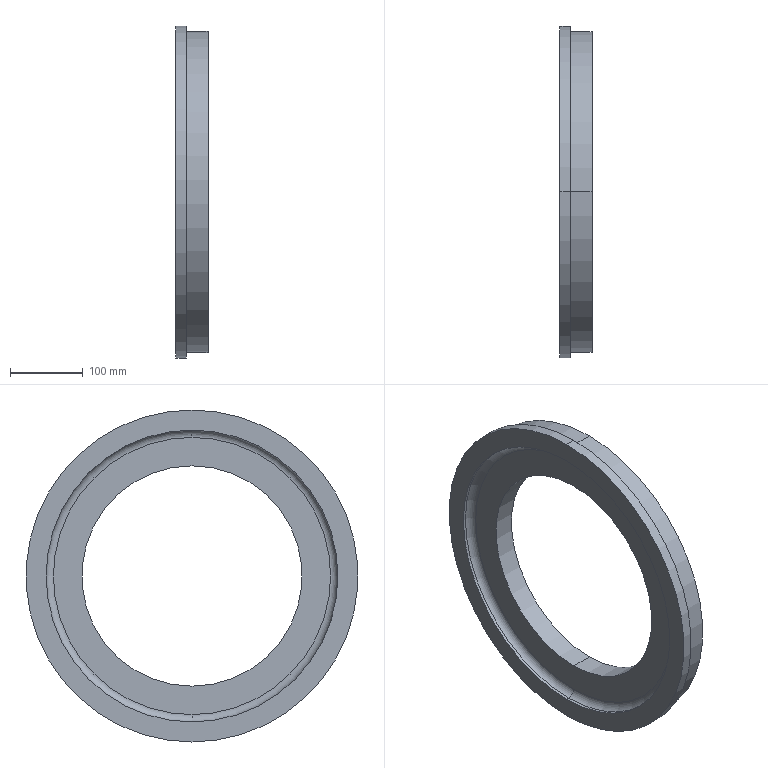Part | SolidWorks | features Fillet 1, Revolution 1 | 1 solid | 26 faces | box 44 x 455 x 455 mm | volume 2505652 mm3 | cylinder 16 | plane 8 | torus 2 | commonest cylinder face diameters 302 x2 326 x2 354 x2 378 x2 400 x2 406 x2
STEP:
#1=CARTESIAN_POINT('',(4.,0.,200.));
#2=VERTEX_POINT('',#1);
#3=CARTESIAN_POINT('',(4.,0.,-200.));
#4=VERTEX_POINT('',#3);
#5=CARTESIAN_POINT('',(4.,0.,0.));
#6=DIRECTION('',(1.,0.,0.));
#7=DIRECTION('',(0.,0.,-1.));
#8=AXIS2_PLACEMENT_3D('',#5,#6,#7);
#9=CIRCLE('',#8,200.);
#10=EDGE_CURVE('',#2,#4,#9,.T.);
#11=ORIENTED_EDGE('',*,*,#10,.F.);
#12=CARTESIAN_POINT('',(14.,0.,190.));
#13=VERTEX_POINT('',#12);
#14=CARTESIAN_POINT('',(4.,0.,190.));
#15=DIRECTION('',(0.,1.,0.));
#16=DIRECTION('',(0.,0.,1.));
#17=AXIS2_PLACEMENT_3D('',#14,#15,#16);
#18=CIRCLE('',#17,10.);
#19=EDGE_CURVE('',#2,#13,#18,.T.);
#20=ORIENTED_EDGE('',*,*,#19,.T.);
#21=CARTESIAN_POINT('',(14.,0.,-190.));
#22=VERTEX_POINT('',#21);
#23=CARTESIAN_POINT('',(14.,0.,0.));
#24=DIRECTION('',(-1.,0.,0.));
#25=DIRECTION('',(0.,0.,-1.));
#26=AXIS2_PLACEMENT_3D('',#23,#24,#25);
#27=CIRCLE('',#26,190.);
#28=EDGE_CURVE('',#22,#13,#27,.T.);
#29=ORIENTED_EDGE('',*,*,#28,.F.);
#30=CARTESIAN_POINT('',(4.,0.,-190.));
#31=DIRECTION('',(0.,-1.,0.));
#32=DIRECTION('',(0.,0.,-1.));
#33=AXIS2_PLACEMENT_3D('',#30,#31,#32);
#34=CIRCLE('',#33,10.);
#35=EDGE_CURVE('',#4,#22,#34,.T.);
#36=ORIENTED_EDGE('',*,*,#35,.F.);
#37=EDGE_LOOP('',(#11,#20,#29,#36));
#38=FACE_OUTER_BOUND('',#37,.T.);
#39=CARTESIAN_POINT('',(4.,0.,0.));
#40=DIRECTION('',(1.,0.,0.));
#41=DIRECTION('',(0.,0.,-1.));
#42=AXIS2_PLACEMENT_3D('',#39,#40,#41);
#43=TOROIDAL_SURFACE('',#42,190.,10.);
#44=ADVANCED_FACE('',(#38),#43,.F.);
#45=CARTESIAN_POINT('',(44.,0.,-151.));
#46=VERTEX_POINT('',#45);
#47=CARTESIAN_POINT('',(44.,0.,151.));
#48=VERTEX_POINT('',#47);
#49=CARTESIAN_POINT('',(44.,0.,0.));
#50=DIRECTION('',(-1.,0.,0.));
#51=DIRECTION('',(0.,0.,1.));
#52=AXIS2_PLACEMENT_3D('',#49,#50,#51);
#53=CIRCLE('',#52,151.);
#54=EDGE_CURVE('',#46,#48,#53,.T.);
#55=ORIENTED_EDGE('',*,*,#54,.F.);
#56=CARTESIAN_POINT('',(14.,0.,-151.));
#57=VERTEX_POINT('',#56);
#58=CARTESIAN_POINT('',(0.,0.,-151.));
#59=DIRECTION('',(-1.,0.,0.));
#60=VECTOR('',#59,1000.);
#61=LINE('',#58,#60);
#62=EDGE_CURVE('',#46,#57,#61,.T.);
#63=ORIENTED_EDGE('',*,*,#62,.T.);
#64=CARTESIAN_POINT('',(14.,0.,151.));
#65=VERTEX_POINT('',#64);
#66=CARTESIAN_POINT('',(14.,0.,0.));
#67=DIRECTION('',(-1.,0.,0.));
#68=DIRECTION('',(0.,0.,1.));
#69=AXIS2_PLACEMENT_3D('',#66,#67,#68);
#70=CIRCLE('',#69,151.);
#71=EDGE_CURVE('',#57,#65,#70,.T.);
#72=ORIENTED_EDGE('',*,*,#71,.T.);
#73=CARTESIAN_POINT('',(0.,0.,151.));
#74=DIRECTION('',(-1.,0.,0.));
#75=VECTOR('',#74,1000.);
#76=LINE('',#73,#75);
#77=EDGE_CURVE('',#48,#65,#76,.T.);
#78=ORIENTED_EDGE('',*,*,#77,.F.);
#79=EDGE_LOOP('',(#55,#63,#72,#78));
#80=FACE_OUTER_BOUND('',#79,.T.);
#81=CARTESIAN_POINT('',(0.,0.,0.));
#82=DIRECTION('',(-1.,0.,0.));
#83=DIRECTION('',(0.,0.,1.));
#84=AXIS2_PLACEMENT_3D('',#81,#82,#83);
#85=CYLINDRICAL_SURFACE('',#84,151.);
#86=ADVANCED_FACE('',(#80),#85,.F.);
#87=CARTESIAN_POINT('',(44.,0.,163.));
#88=VERTEX_POINT('',#87);
#89=CARTESIAN_POINT('',(44.,0.,-163.));
#90=VERTEX_POINT('',#89);
#91=CARTESIAN_POINT('',(44.,0.,0.));
#92=DIRECTION('',(-1.,0.,0.));
#93=DIRECTION('',(0.,0.,1.));
#94=AXIS2_PLACEMENT_3D('',#91,#92,#93);
#95=CIRCLE('',#94,163.);
#96=EDGE_CURVE('',#88,#90,#95,.T.);
#97=ORIENTED_EDGE('',*,*,#96,.T.);
#98=CARTESIAN_POINT('',(30.,0.,-163.));
#99=VERTEX_POINT('',#98);
#100=CARTESIAN_POINT('',(0.,0.,-163.));
#101=DIRECTION('',(-1.,0.,0.));
#102=VECTOR('',#101,1000.);
#103=LINE('',#100,#102);
#104=EDGE_CURVE('',#90,#99,#103,.T.);
#105=ORIENTED_EDGE('',*,*,#104,.T.);
#106=CARTESIAN_POINT('',(30.,0.,163.));
#107=VERTEX_POINT('',#106);
#108=CARTESIAN_POINT('',(30.,0.,0.));
#109=DIRECTION('',(-1.,0.,0.));
#110=DIRECTION('',(0.,0.,1.));
#111=AXIS2_PLACEMENT_3D('',#108,#109,#110);
#112=CIRCLE('',#111,163.);
#113=EDGE_CURVE('',#107,#99,#112,.T.);
#114=ORIENTED_EDGE('',*,*,#113,.F.);
#115=CARTESIAN_POINT('',(0.,0.,163.));
#116=DIRECTION('',(-1.,0.,0.));
#117=VECTOR('',#116,1000.);
#118=LINE('',#115,#117);
#119=EDGE_CURVE('',#88,#107,#118,.T.);
#120=ORIENTED_EDGE('',*,*,#119,.F.);
#121=EDGE_LOOP('',(#97,#105,#114,#120));
#122=FACE_OUTER_BOUND('',#121,.T.);
#123=CARTESIAN_POINT('',(0.,0.,0.));
#124=DIRECTION('',(-1.,0.,0.));
#125=DIRECTION('',(0.,0.,1.));
#126=AXIS2_PLACEMENT_3D('',#123,#124,#125);
#127=CYLINDRICAL_SURFACE('',#126,163.);
#128=ADVANCED_FACE('',(#122),#127,.T.);
#129=CARTESIAN_POINT('',(44.,0.,-177.));
#130=VERTEX_POINT('',#129);
#131=CARTESIAN_POINT('',(44.,0.,177.));
#132=VERTEX_POINT('',#131);
#133=CARTESIAN_POINT('',(44.,0.,0.));
#134=DIRECTION('',(-1.,0.,0.));
#135=DIRECTION('',(0.,0.,1.));
#136=AXIS2_PLACEMENT_3D('',#133,#134,#135);
#137=CIRCLE('',#136,177.);
#138=EDGE_CURVE('',#130,#132,#137,.T.);
#139=ORIENTED_EDGE('',*,*,#138,.F.);
#140=CARTESIAN_POINT('',(30.,0.,-177.));
#141=VERTEX_POINT('',#140);
#142=CARTESIAN_POINT('',(0.,0.,-177.));
#143=DIRECTION('',(-1.,0.,0.));
#144=VECTOR('',#143,1000.);
#145=LINE('',#142,#144);
#146=EDGE_CURVE('',#130,#141,#145,.T.);
#147=ORIENTED_EDGE('',*,*,#146,.T.);
#148=CARTESIAN_POINT('',(30.,0.,177.));
#149=VERTEX_POINT('',#148);
#150=CARTESIAN_POINT('',(30.,0.,0.));
#151=DIRECTION('',(-1.,0.,0.));
#152=DIRECTION('',(0.,0.,1.));
#153=AXIS2_PLACEMENT_3D('',#150,#151,#152);
#154=CIRCLE('',#153,177.);
#155=EDGE_CURVE('',#141,#149,#154,.T.);
#156=ORIENTED_EDGE('',*,*,#155,.T.);
#157=CARTESIAN_POINT('',(0.,0.,177.));
#158=DIRECTION('',(-1.,0.,0.));
#159=VECTOR('',#158,1000.);
#160=LINE('',#157,#159);
#161=EDGE_CURVE('',#132,#149,#160,.T.);
#162=ORIENTED_EDGE('',*,*,#161,.F.);
#163=EDGE_LOOP('',(#139,#147,#156,#162));
#164=FACE_OUTER_BOUND('',#163,.T.);
#165=CARTESIAN_POINT('',(0.,0.,0.));
#166=DIRECTION('',(-1.,0.,0.));
#167=DIRECTION('',(0.,0.,1.));
#168=AXIS2_PLACEMENT_3D('',#165,#166,#167);
#169=CYLINDRICAL_SURFACE('',#168,177.);
#170=ADVANCED_FACE('',(#164),#169,.F.);
#171=CARTESIAN_POINT('',(44.,0.,189.));
#172=VERTEX_POINT('',#171);
#173=CARTESIAN_POINT('',(44.,0.,-189.));
#174=VERTEX_POINT('',#173);
#175=CARTESIAN_POINT('',(44.,0.,0.));
#176=DIRECTION('',(-1.,0.,0.));
#177=DIRECTION('',(0.,0.,1.));
#178=AXIS2_PLACEMENT_3D('',#175,#176,#177);
#179=CIRCLE('',#178,189.);
#180=EDGE_CURVE('',#172,#174,#179,.T.);
#181=ORIENTED_EDGE('',*,*,#180,.T.);
#182=CARTESIAN_POINT('',(30.,0.,-189.));
#183=VERTEX_POINT('',#182);
#184=CARTESIAN_POINT('',(0.,0.,-189.));
#185=DIRECTION('',(-1.,0.,0.));
#186=VECTOR('',#185,1000.);
#187=LINE('',#184,#186);
#188=EDGE_CURVE('',#174,#183,#187,.T.);
#189=ORIENTED_EDGE('',*,*,#188,.T.);
#190=CARTESIAN_POINT('',(30.,0.,189.));
#191=VERTEX_POINT('',#190);
#192=CARTESIAN_POINT('',(30.,0.,0.));
#193=DIRECTION('',(-1.,0.,0.));
#194=DIRECTION('',(0.,0.,1.));
#195=AXIS2_PLACEMENT_3D('',#192,#193,#194);
#196=CIRCLE('',#195,189.);
#197=EDGE_CURVE('',#191,#183,#196,.T.);
#198=ORIENTED_EDGE('',*,*,#197,.F.);
#199=CARTESIAN_POINT('',(0.,0.,189.));
#200=DIRECTION('',(-1.,0.,0.));
#201=VECTOR('',#200,1000.);
#202=LINE('',#199,#201);
#203=EDGE_CURVE('',#172,#191,#202,.T.);
#204=ORIENTED_EDGE('',*,*,#203,.F.);
#205=EDGE_LOOP('',(#181,#189,#198,#204));
#206=FACE_OUTER_BOUND('',#205,.T.);
#207=CARTESIAN_POINT('',(0.,0.,0.));
#208=DIRECTION('',(-1.,0.,0.));
#209=DIRECTION('',(0.,0.,1.));
#210=AXIS2_PLACEMENT_3D('',#207,#208,#209);
#211=CYLINDRICAL_SURFACE('',#210,189.);
#212=ADVANCED_FACE('',(#206),#211,.T.);
#213=CARTESIAN_POINT('',(44.,0.,-203.));
#214=VERTEX_POINT('',#213);
#215=CARTESIAN_POINT('',(44.,0.,203.));
#216=VERTEX_POINT('',#215);
#217=CARTESIAN_POINT('',(44.,0.,0.));
#218=DIRECTION('',(-1.,0.,0.));
#219=DIRECTION('',(0.,0.,1.));
#220=AXIS2_PLACEMENT_3D('',#217,#218,#219);
#221=CIRCLE('',#220,203.);
#222=EDGE_CURVE('',#214,#216,#221,.T.);
#223=ORIENTED_EDGE('',*,*,#222,.F.);
#224=CARTESIAN_POINT('',(30.,0.,-203.));
#225=VERTEX_POINT('',#224);
#226=CARTESIAN_POINT('',(0.,0.,-203.));
#227=DIRECTION('',(-1.,0.,0.));
#228=VECTOR('',#227,1000.);
#229=LINE('',#226,#228);
#230=EDGE_CURVE('',#214,#225,#229,.T.);
#231=ORIENTED_EDGE('',*,*,#230,.T.);
#232=CARTESIAN_POINT('',(30.,0.,203.));
#233=VERTEX_POINT('',#232);
#234=CARTESIAN_POINT('',(30.,0.,0.));
#235=DIRECTION('',(-1.,0.,0.));
#236=DIRECTION('',(0.,0.,1.));
#237=AXIS2_PLACEMENT_3D('',#234,#235,#236);
#238=CIRCLE('',#237,203.);
#239=EDGE_CURVE('',#225,#233,#238,.T.);
#240=ORIENTED_EDGE('',*,*,#239,.T.);
#241=CARTESIAN_POINT('',(0.,0.,203.));
#242=DIRECTION('',(-1.,0.,0.));
#243=VECTOR('',#242,1000.);
#244=LINE('',#241,#243);
#245=EDGE_CURVE('',#216,#233,#244,.T.);
#246=ORIENTED_EDGE('',*,*,#245,.F.);
#247=EDGE_LOOP('',(#223,#231,#240,#246));
#248=FACE_OUTER_BOUND('',#247,.T.);
#249=CARTESIAN_POINT('',(0.,0.,0.));
#250=DIRECTION('',(-1.,0.,0.));
#251=DIRECTION('',(0.,0.,1.));
#252=AXIS2_PLACEMENT_3D('',#249,#250,#251);
#253=CYLINDRICAL_SURFACE('',#252,203.);
#254=ADVANCED_FACE('',(#248),#253,.F.);
#255=CARTESIAN_POINT('',(44.,0.,220.));
#256=VERTEX_POINT('',#255);
#257=CARTESIAN_POINT('',(44.,0.,-220.));
#258=VERTEX_POINT('',#257);
#259=CARTESIAN_POINT('',(44.,0.,0.));
#260=DIRECTION('',(-1.,0.,0.));
#261=DIRECTION('',(0.,0.,1.));
#262=AXIS2_PLACEMENT_3D('',#259,#260,#261);
#263=CIRCLE('',#262,220.);
#264=EDGE_CURVE('',#256,#258,#263,.T.);
#265=ORIENTED_EDGE('',*,*,#264,.T.);
#266=CARTESIAN_POINT('',(14.,0.,-220.));
#267=VERTEX_POINT('',#266);
#268=CARTESIAN_POINT('',(0.,0.,-220.));
#269=DIRECTION('',(-1.,0.,0.));
#270=VECTOR('',#269,1000.);
#271=LINE('',#268,#270);
#272=EDGE_CURVE('',#258,#267,#271,.T.);
#273=ORIENTED_EDGE('',*,*,#272,.T.);
#274=CARTESIAN_POINT('',(14.,0.,220.));
#275=VERTEX_POINT('',#274);
#276=CARTESIAN_POINT('',(14.,0.,0.));
#277=DIRECTION('',(-1.,0.,0.));
#278=DIRECTION('',(0.,0.,1.));
#279=AXIS2_PLACEMENT_3D('',#276,#277,#278);
#280=CIRCLE('',#279,220.);
#281=EDGE_CURVE('',#275,#267,#280,.T.);
#282=ORIENTED_EDGE('',*,*,#281,.F.);
#283=CARTESIAN_POINT('',(0.,0.,220.));
#284=DIRECTION('',(-1.,0.,0.));
#285=VECTOR('',#284,1000.);
#286=LINE('',#283,#285);
#287=EDGE_CURVE('',#256,#275,#286,.T.);
#288=ORIENTED_EDGE('',*,*,#287,.F.);
#289=EDGE_LOOP('',(#265,#273,#282,#288));
#290=FACE_OUTER_BOUND('',#289,.T.);
#291=CARTESIAN_POINT('',(0.,0.,0.));
#292=DIRECTION('',(-1.,0.,0.));
#293=DIRECTION('',(0.,0.,1.));
#294=AXIS2_PLACEMENT_3D('',#291,#292,#293);
#295=CYLINDRICAL_SURFACE('',#294,220.);
#296=ADVANCED_FACE('',(#290),#295,.T.);
#297=CARTESIAN_POINT('',(14.,0.,227.5));
#298=VERTEX_POINT('',#297);
#299=CARTESIAN_POINT('',(14.,0.,-227.5));
#300=VERTEX_POINT('',#299);
#301=CARTESIAN_POINT('',(14.,0.,0.));
#302=DIRECTION('',(-1.,0.,0.));
#303=DIRECTION('',(0.,0.,1.));
#304=AXIS2_PLACEMENT_3D('',#301,#302,#303);
#305=CIRCLE('',#304,227.5);
#306=EDGE_CURVE('',#298,#300,#305,.T.);
#307=ORIENTED_EDGE('',*,*,#306,.T.);
#308=CARTESIAN_POINT('',(0.,0.,-227.5));
#309=VERTEX_POINT('',#308);
#310=CARTESIAN_POINT('',(0.,0.,-227.5));
#311=DIRECTION('',(-1.,0.,0.));
#312=VECTOR('',#311,1000.);
#313=LINE('',#310,#312);
#314=EDGE_CURVE('',#300,#309,#313,.T.);
#315=ORIENTED_EDGE('',*,*,#314,.T.);
#316=CARTESIAN_POINT('',(0.,0.,227.5));
#317=VERTEX_POINT('',#316);
#318=CARTESIAN_POINT('',(0.,0.,0.));
#319=DIRECTION('',(-1.,0.,0.));
#320=DIRECTION('',(0.,0.,1.));
#321=AXIS2_PLACEMENT_3D('',#318,#319,#320);
#322=CIRCLE('',#321,227.5);
#323=EDGE_CURVE('',#317,#309,#322,.T.);
#324=ORIENTED_EDGE('',*,*,#323,.F.);
#325=CARTESIAN_POINT('',(0.,0.,227.5));
#326=DIRECTION('',(-1.,0.,0.));
#327=VECTOR('',#326,1000.);
#328=LINE('',#325,#327);
#329=EDGE_CURVE('',#298,#317,#328,.T.);
#330=ORIENTED_EDGE('',*,*,#329,.F.);
#331=EDGE_LOOP('',(#307,#315,#324,#330));
#332=FACE_OUTER_BOUND('',#331,.T.);
#333=CARTESIAN_POINT('',(0.,0.,0.));
#334=DIRECTION('',(-1.,0.,0.));
#335=DIRECTION('',(0.,0.,1.));
#336=AXIS2_PLACEMENT_3D('',#333,#334,#335);
#337=CYLINDRICAL_SURFACE('',#336,227.5);
#338=ADVANCED_FACE('',(#332),#337,.T.);
#339=ORIENTED_EDGE('',*,*,#10,.T.);
#340=CARTESIAN_POINT('',(0.,0.,-200.));
#341=VERTEX_POINT('',#340);
#342=CARTESIAN_POINT('',(0.,0.,-200.));
#343=DIRECTION('',(-1.,0.,0.));
#344=VECTOR('',#343,1000.);
#345=LINE('',#342,#344);
#346=EDGE_CURVE('',#4,#341,#345,.T.);
#347=ORIENTED_EDGE('',*,*,#346,.T.);
#348=CARTESIAN_POINT('',(0.,0.,200.));
#349=VERTEX_POINT('',#348);
#350=CARTESIAN_POINT('',(0.,0.,0.));
#351=DIRECTION('',(-1.,0.,0.));
#352=DIRECTION('',(0.,0.,1.));
#353=AXIS2_PLACEMENT_3D('',#350,#351,#352);
#354=CIRCLE('',#353,200.);
#355=EDGE_CURVE('',#341,#349,#354,.T.);
#356=ORIENTED_EDGE('',*,*,#355,.T.);
#357=CARTESIAN_POINT('',(0.,0.,200.));
#358=DIRECTION('',(-1.,0.,0.));
#359=VECTOR('',#358,1000.);
#360=LINE('',#357,#359);
#361=EDGE_CURVE('',#2,#349,#360,.T.);
#362=ORIENTED_EDGE('',*,*,#361,.F.);
#363=EDGE_LOOP('',(#339,#347,#356,#362));
#364=FACE_OUTER_BOUND('',#363,.T.);
#365=CARTESIAN_POINT('',(0.,0.,0.));
#366=DIRECTION('',(-1.,0.,0.));
#367=DIRECTION('',(0.,0.,1.));
#368=AXIS2_PLACEMENT_3D('',#365,#366,#367);
#369=CYLINDRICAL_SURFACE('',#368,200.);
#370=ADVANCED_FACE('',(#364),#369,.F.);
#371=ORIENTED_EDGE('',*,*,#346,.F.);
#372=CARTESIAN_POINT('',(4.,0.,0.));
#373=DIRECTION('',(1.,0.,0.));
#374=DIRECTION('',(0.,0.,-1.));
#375=AXIS2_PLACEMENT_3D('',#372,#373,#374);
#376=CIRCLE('',#375,200.);
#377=EDGE_CURVE('',#4,#2,#376,.T.);
#378=ORIENTED_EDGE('',*,*,#377,.T.);
#379=ORIENTED_EDGE('',*,*,#361,.T.);
#380=CARTESIAN_POINT('',(0.,0.,0.));
#381=DIRECTION('',(-1.,0.,0.));
#382=DIRECTION('',(0.,0.,1.));
#383=AXIS2_PLACEMENT_3D('',#380,#381,#382);
#384=CIRCLE('',#383,200.);
#385=EDGE_CURVE('',#349,#341,#384,.T.);
#386=ORIENTED_EDGE('',*,*,#385,.T.);
#387=EDGE_LOOP('',(#371,#378,#379,#386));
#388=FACE_OUTER_BOUND('',#387,.T.);
#389=CARTESIAN_POINT('',(0.,0.,0.));
#390=DIRECTION('',(-1.,0.,0.));
#391=DIRECTION('',(0.,0.,1.));
#392=AXIS2_PLACEMENT_3D('',#389,#390,#391);
#393=CYLINDRICAL_SURFACE('',#392,200.);
#394=ADVANCED_FACE('',(#388),#393,.F.);
#395=ORIENTED_EDGE('',*,*,#385,.F.);
#396=ORIENTED_EDGE('',*,*,#355,.F.);
#397=EDGE_LOOP('',(#395,#396));
#398=FACE_BOUND('',#397,.T.);
#399=ORIENTED_EDGE('',*,*,#323,.T.);
#400=CARTESIAN_POINT('',(0.,0.,0.));
#401=DIRECTION('',(-1.,0.,0.));
#402=DIRECTION('',(0.,0.,1.));
#403=AXIS2_PLACEMENT_3D('',#400,#401,#402);
#404=CIRCLE('',#403,227.5);
#405=EDGE_CURVE('',#309,#317,#404,.T.);
#406=ORIENTED_EDGE('',*,*,#405,.T.);
#407=EDGE_LOOP('',(#399,#406));
#408=FACE_OUTER_BOUND('',#407,.T.);
#409=CARTESIAN_POINT('',(0.,0.,-200.));
#410=DIRECTION('',(1.,0.,0.));
#411=DIRECTION('',(0.,0.,-1.));
#412=AXIS2_PLACEMENT_3D('',#409,#410,#411);
#413=PLANE('',#412);
#414=ADVANCED_FACE('',(#398,#408),#413,.F.);
#415=ORIENTED_EDGE('',*,*,#314,.F.);
#416=CARTESIAN_POINT('',(14.,0.,0.));
#417=DIRECTION('',(-1.,0.,0.));
#418=DIRECTION('',(0.,0.,1.));
#419=AXIS2_PLACEMENT_3D('',#416,#417,#418);
#420=CIRCLE('',#419,227.5);
#421=EDGE_CURVE('',#300,#298,#420,.T.);
#422=ORIENTED_EDGE('',*,*,#421,.T.);
#423=ORIENTED_EDGE('',*,*,#329,.T.);
#424=ORIENTED_EDGE('',*,*,#405,.F.);
#425=EDGE_LOOP('',(#415,#422,#423,#424));
#426=FACE_OUTER_BOUND('',#425,.T.);
#427=CARTESIAN_POINT('',(0.,0.,0.));
#428=DIRECTION('',(-1.,0.,0.));
#429=DIRECTION('',(0.,0.,1.));
#430=AXIS2_PLACEMENT_3D('',#427,#428,#429);
#431=CYLINDRICAL_SURFACE('',#430,227.5);
#432=ADVANCED_FACE('',(#426),#431,.T.);
#433=ORIENTED_EDGE('',*,*,#306,.F.);
#434=ORIENTED_EDGE('',*,*,#421,.F.);
#435=EDGE_LOOP('',(#433,#434));
#436=FACE_OUTER_BOUND('',#435,.T.);
#437=ORIENTED_EDGE('',*,*,#281,.T.);
#438=CARTESIAN_POINT('',(14.,0.,0.));
#439=DIRECTION('',(-1.,0.,0.));
#440=DIRECTION('',(0.,0.,1.));
#441=AXIS2_PLACEMENT_3D('',#438,#439,#440);
#442=CIRCLE('',#441,220.);
#443=EDGE_CURVE('',#267,#275,#442,.T.);
#444=ORIENTED_EDGE('',*,*,#443,.T.);
#445=EDGE_LOOP('',(#437,#444));
#446=FACE_BOUND('',#445,.T.);
#447=CARTESIAN_POINT('',(14.,0.,-227.5));
#448=DIRECTION('',(-1.,0.,0.));
#449=DIRECTION('',(0.,0.,1.));
#450=AXIS2_PLACEMENT_3D('',#447,#448,#449);
#451=PLANE('',#450);
#452=ADVANCED_FACE('',(#436,#446),#451,.F.);
#453=ORIENTED_EDGE('',*,*,#272,.F.);
#454=CARTESIAN_POINT('',(44.,0.,0.));
#455=DIRECTION('',(-1.,0.,0.));
#456=DIRECTION('',(0.,0.,1.));
#457=AXIS2_PLACEMENT_3D('',#454,#455,#456);
#458=CIRCLE('',#457,220.);
#459=EDGE_CURVE('',#258,#256,#458,.T.);
#460=ORIENTED_EDGE('',*,*,#459,.T.);
#461=ORIENTED_EDGE('',*,*,#287,.T.);
#462=ORIENTED_EDGE('',*,*,#443,.F.);
#463=EDGE_LOOP('',(#453,#460,#461,#462));
#464=FACE_OUTER_BOUND('',#463,.T.);
#465=CARTESIAN_POINT('',(0.,0.,0.));
#466=DIRECTION('',(-1.,0.,0.));
#467=DIRECTION('',(0.,0.,1.));
#468=AXIS2_PLACEMENT_3D('',#465,#466,#467);
#469=CYLINDRICAL_SURFACE('',#468,220.);
#470=ADVANCED_FACE('',(#464),#469,.T.);
#471=ORIENTED_EDGE('',*,*,#264,.F.);
#472=ORIENTED_EDGE('',*,*,#459,.F.);
#473=EDGE_LOOP('',(#471,#472));
#474=FACE_OUTER_BOUND('',#473,.T.);
#475=CARTESIAN_POINT('',(44.,0.,0.));
#476=DIRECTION('',(-1.,0.,0.));
#477=DIRECTION('',(0.,0.,1.));
#478=AXIS2_PLACEMENT_3D('',#475,#476,#477);
#479=CIRCLE('',#478,203.);
#480=EDGE_CURVE('',#216,#214,#479,.T.);
#481=ORIENTED_EDGE('',*,*,#480,.T.);
#482=ORIENTED_EDGE('',*,*,#222,.T.);
#483=EDGE_LOOP('',(#481,#482));
#484=FACE_BOUND('',#483,.T.);
#485=CARTESIAN_POINT('',(44.,0.,-220.));
#486=DIRECTION('',(-1.,0.,0.));
#487=DIRECTION('',(0.,0.,1.));
#488=AXIS2_PLACEMENT_3D('',#485,#486,#487);
#489=PLANE('',#488);
#490=ADVANCED_FACE('',(#474,#484),#489,.F.);
#491=ORIENTED_EDGE('',*,*,#230,.F.);
#492=ORIENTED_EDGE('',*,*,#480,.F.);
#493=ORIENTED_EDGE('',*,*,#245,.T.);
#494=CARTESIAN_POINT('',(30.,0.,0.));
#495=DIRECTION('',(-1.,0.,0.));
#496=DIRECTION('',(0.,0.,1.));
#497=AXIS2_PLACEMENT_3D('',#494,#495,#496);
#498=CIRCLE('',#497,203.);
#499=EDGE_CURVE('',#233,#225,#498,.T.);
#500=ORIENTED_EDGE('',*,*,#499,.T.);
#501=EDGE_LOOP('',(#491,#492,#493,#500));
#502=FACE_OUTER_BOUND('',#501,.T.);
#503=CARTESIAN_POINT('',(0.,0.,0.));
#504=DIRECTION('',(-1.,0.,0.));
#505=DIRECTION('',(0.,0.,1.));
#506=AXIS2_PLACEMENT_3D('',#503,#504,#505);
#507=CYLINDRICAL_SURFACE('',#506,203.);
#508=ADVANCED_FACE('',(#502),#507,.F.);
#509=ORIENTED_EDGE('',*,*,#499,.F.);
#510=ORIENTED_EDGE('',*,*,#239,.F.);
#511=EDGE_LOOP('',(#509,#510));
#512=FACE_OUTER_BOUND('',#511,.T.);
#513=ORIENTED_EDGE('',*,*,#197,.T.);
#514=CARTESIAN_POINT('',(30.,0.,0.));
#515=DIRECTION('',(-1.,0.,0.));
#516=DIRECTION('',(0.,0.,1.));
#517=AXIS2_PLACEMENT_3D('',#514,#515,#516);
#518=CIRCLE('',#517,189.);
#519=EDGE_CURVE('',#183,#191,#518,.T.);
#520=ORIENTED_EDGE('',*,*,#519,.T.);
#521=EDGE_LOOP('',(#513,#520));
#522=FACE_BOUND('',#521,.T.);
#523=CARTESIAN_POINT('',(30.,0.,-203.));
#524=DIRECTION('',(-1.,0.,0.));
#525=DIRECTION('',(0.,0.,1.));
#526=AXIS2_PLACEMENT_3D('',#523,#524,#525);
#527=PLANE('',#526);
#528=ADVANCED_FACE('',(#512,#522),#527,.F.);
#529=ORIENTED_EDGE('',*,*,#188,.F.);
#530=CARTESIAN_POINT('',(44.,0.,0.));
#531=DIRECTION('',(-1.,0.,0.));
#532=DIRECTION('',(0.,0.,1.));
#533=AXIS2_PLACEMENT_3D('',#530,#531,#532);
#534=CIRCLE('',#533,189.);
#535=EDGE_CURVE('',#174,#172,#534,.T.);
#536=ORIENTED_EDGE('',*,*,#535,.T.);
#537=ORIENTED_EDGE('',*,*,#203,.T.);
#538=ORIENTED_EDGE('',*,*,#519,.F.);
#539=EDGE_LOOP('',(#529,#536,#537,#538));
#540=FACE_OUTER_BOUND('',#539,.T.);
#541=CARTESIAN_POINT('',(0.,0.,0.));
#542=DIRECTION('',(-1.,0.,0.));
#543=DIRECTION('',(0.,0.,1.));
#544=AXIS2_PLACEMENT_3D('',#541,#542,#543);
#545=CYLINDRICAL_SURFACE('',#544,189.);
#546=ADVANCED_FACE('',(#540),#545,.T.);
#547=ORIENTED_EDGE('',*,*,#180,.F.);
#548=ORIENTED_EDGE('',*,*,#535,.F.);
#549=EDGE_LOOP('',(#547,#548));
#550=FACE_OUTER_BOUND('',#549,.T.);
#551=CARTESIAN_POINT('',(44.,0.,0.));
#552=DIRECTION('',(-1.,0.,0.));
#553=DIRECTION('',(0.,0.,1.));
#554=AXIS2_PLACEMENT_3D('',#551,#552,#553);
#555=CIRCLE('',#554,177.);
#556=EDGE_CURVE('',#132,#130,#555,.T.);
#557=ORIENTED_EDGE('',*,*,#556,.T.);
#558=ORIENTED_EDGE('',*,*,#138,.T.);
#559=EDGE_LOOP('',(#557,#558));
#560=FACE_BOUND('',#559,.T.);
#561=CARTESIAN_POINT('',(44.,0.,-189.));
#562=DIRECTION('',(-1.,0.,0.));
#563=DIRECTION('',(0.,0.,1.));
#564=AXIS2_PLACEMENT_3D('',#561,#562,#563);
#565=PLANE('',#564);
#566=ADVANCED_FACE('',(#550,#560),#565,.F.);
#567=ORIENTED_EDGE('',*,*,#146,.F.);
#568=ORIENTED_EDGE('',*,*,#556,.F.);
#569=ORIENTED_EDGE('',*,*,#161,.T.);
#570=CARTESIAN_POINT('',(30.,0.,0.));
#571=DIRECTION('',(-1.,0.,0.));
#572=DIRECTION('',(0.,0.,1.));
#573=AXIS2_PLACEMENT_3D('',#570,#571,#572);
#574=CIRCLE('',#573,177.);
#575=EDGE_CURVE('',#149,#141,#574,.T.);
#576=ORIENTED_EDGE('',*,*,#575,.T.);
#577=EDGE_LOOP('',(#567,#568,#569,#576));
#578=FACE_OUTER_BOUND('',#577,.T.);
#579=CARTESIAN_POINT('',(0.,0.,0.));
#580=DIRECTION('',(-1.,0.,0.));
#581=DIRECTION('',(0.,0.,1.));
#582=AXIS2_PLACEMENT_3D('',#579,#580,#581);
#583=CYLINDRICAL_SURFACE('',#582,177.);
#584=ADVANCED_FACE('',(#578),#583,.F.);
#585=ORIENTED_EDGE('',*,*,#575,.F.);
#586=ORIENTED_EDGE('',*,*,#155,.F.);
#587=EDGE_LOOP('',(#585,#586));
#588=FACE_OUTER_BOUND('',#587,.T.);
#589=ORIENTED_EDGE('',*,*,#113,.T.);
#590=CARTESIAN_POINT('',(30.,0.,0.));
#591=DIRECTION('',(-1.,0.,0.));
#592=DIRECTION('',(0.,0.,1.));
#593=AXIS2_PLACEMENT_3D('',#590,#591,#592);
#594=CIRCLE('',#593,163.);
#595=EDGE_CURVE('',#99,#107,#594,.T.);
#596=ORIENTED_EDGE('',*,*,#595,.T.);
#597=EDGE_LOOP('',(#589,#596));
#598=FACE_BOUND('',#597,.T.);
#599=CARTESIAN_POINT('',(30.,0.,-177.));
#600=DIRECTION('',(-1.,0.,0.));
#601=DIRECTION('',(0.,0.,1.));
#602=AXIS2_PLACEMENT_3D('',#599,#600,#601);
#603=PLANE('',#602);
#604=ADVANCED_FACE('',(#588,#598),#603,.F.);
#605=ORIENTED_EDGE('',*,*,#104,.F.);
#606=CARTESIAN_POINT('',(44.,0.,0.));
#607=DIRECTION('',(-1.,0.,0.));
#608=DIRECTION('',(0.,0.,1.));
#609=AXIS2_PLACEMENT_3D('',#606,#607,#608);
#610=CIRCLE('',#609,163.);
#611=EDGE_CURVE('',#90,#88,#610,.T.);
#612=ORIENTED_EDGE('',*,*,#611,.T.);
#613=ORIENTED_EDGE('',*,*,#119,.T.);
#614=ORIENTED_EDGE('',*,*,#595,.F.);
#615=EDGE_LOOP('',(#605,#612,#613,#614));
#616=FACE_OUTER_BOUND('',#615,.T.);
#617=CARTESIAN_POINT('',(0.,0.,0.));
#618=DIRECTION('',(-1.,0.,0.));
#619=DIRECTION('',(0.,0.,1.));
#620=AXIS2_PLACEMENT_3D('',#617,#618,#619);
#621=CYLINDRICAL_SURFACE('',#620,163.);
#622=ADVANCED_FACE('',(#616),#621,.T.);
#623=ORIENTED_EDGE('',*,*,#96,.F.);
#624=ORIENTED_EDGE('',*,*,#611,.F.);
#625=EDGE_LOOP('',(#623,#624));
#626=FACE_OUTER_BOUND('',#625,.T.);
#627=CARTESIAN_POINT('',(44.,0.,0.));
#628=DIRECTION('',(-1.,0.,0.));
#629=DIRECTION('',(0.,0.,1.));
#630=AXIS2_PLACEMENT_3D('',#627,#628,#629);
#631=CIRCLE('',#630,151.);
#632=EDGE_CURVE('',#48,#46,#631,.T.);
#633=ORIENTED_EDGE('',*,*,#632,.T.);
#634=ORIENTED_EDGE('',*,*,#54,.T.);
#635=EDGE_LOOP('',(#633,#634));
#636=FACE_BOUND('',#635,.T.);
#637=CARTESIAN_POINT('',(44.,0.,-163.));
#638=DIRECTION('',(-1.,0.,0.));
#639=DIRECTION('',(0.,0.,1.));
#640=AXIS2_PLACEMENT_3D('',#637,#638,#639);
#641=PLANE('',#640);
#642=ADVANCED_FACE('',(#626,#636),#641,.F.);
#643=ORIENTED_EDGE('',*,*,#62,.F.);
#644=ORIENTED_EDGE('',*,*,#632,.F.);
#645=ORIENTED_EDGE('',*,*,#77,.T.);
#646=CARTESIAN_POINT('',(14.,0.,0.));
#647=DIRECTION('',(-1.,0.,0.));
#648=DIRECTION('',(0.,0.,1.));
#649=AXIS2_PLACEMENT_3D('',#646,#647,#648);
#650=CIRCLE('',#649,151.);
#651=EDGE_CURVE('',#65,#57,#650,.T.);
#652=ORIENTED_EDGE('',*,*,#651,.T.);
#653=EDGE_LOOP('',(#643,#644,#645,#652));
#654=FACE_OUTER_BOUND('',#653,.T.);
#655=CARTESIAN_POINT('',(0.,0.,0.));
#656=DIRECTION('',(-1.,0.,0.));
#657=DIRECTION('',(0.,0.,1.));
#658=AXIS2_PLACEMENT_3D('',#655,#656,#657);
#659=CYLINDRICAL_SURFACE('',#658,151.);
#660=ADVANCED_FACE('',(#654),#659,.F.);
#661=ORIENTED_EDGE('',*,*,#28,.T.);
#662=CARTESIAN_POINT('',(14.,0.,0.));
#663=DIRECTION('',(-1.,0.,0.));
#664=DIRECTION('',(0.,0.,-1.));
#665=AXIS2_PLACEMENT_3D('',#662,#663,#664);
#666=CIRCLE('',#665,190.);
#667=EDGE_CURVE('',#13,#22,#666,.T.);
#668=ORIENTED_EDGE('',*,*,#667,.T.);
#669=EDGE_LOOP('',(#661,#668));
#670=FACE_OUTER_BOUND('',#669,.T.);
#671=ORIENTED_EDGE('',*,*,#651,.F.);
#672=ORIENTED_EDGE('',*,*,#71,.F.);
#673=EDGE_LOOP('',(#671,#672));
#674=FACE_BOUND('',#673,.T.);
#675=CARTESIAN_POINT('',(14.,0.,-151.));
#676=DIRECTION('',(1.,0.,0.));
#677=DIRECTION('',(0.,0.,-1.));
#678=AXIS2_PLACEMENT_3D('',#675,#676,#677);
#679=PLANE('',#678);
#680=ADVANCED_FACE('',(#670,#674),#679,.F.);
#681=ORIENTED_EDGE('',*,*,#19,.F.);
#682=ORIENTED_EDGE('',*,*,#377,.F.);
#683=ORIENTED_EDGE('',*,*,#35,.T.);
#684=ORIENTED_EDGE('',*,*,#667,.F.);
#685=EDGE_LOOP('',(#681,#682,#683,#684));
#686=FACE_OUTER_BOUND('',#685,.T.);
#687=CARTESIAN_POINT('',(4.,0.,0.));
#688=DIRECTION('',(1.,0.,0.));
#689=DIRECTION('',(0.,0.,-1.));
#690=AXIS2_PLACEMENT_3D('',#687,#688,#689);
#691=TOROIDAL_SURFACE('',#690,190.,10.);
#692=ADVANCED_FACE('',(#686),#691,.F.);
#693=CLOSED_SHELL('',(#44,#86,#128,#170,#212,#254,#296,#338,#370,#394,#414,#432,#452,#470,#490,#508,#528,#546,#566,#584,#604,#622,#642,#660,#680,#692));
#694=MANIFOLD_SOLID_BREP('',#693);
#695=CARTESIAN_POINT('',(0.,0.,0.));
#696=DIRECTION('',(0.,0.,1.));
#697=DIRECTION('',(1.,0.,0.));
#698=AXIS2_PLACEMENT_3D('',#695,#696,#697);
#699=(LENGTH_UNIT()NAMED_UNIT(*)SI_UNIT(.MILLI.,.METRE.));
#700=UNCERTAINTY_MEASURE_WITH_UNIT(LENGTH_MEASURE(0.00001),#699,'','');
#701=(NAMED_UNIT(*)PLANE_ANGLE_UNIT()SI_UNIT($,.RADIAN.));
#702=(NAMED_UNIT(*)SI_UNIT($,.STERADIAN.)SOLID_ANGLE_UNIT());
#703=(GEOMETRIC_REPRESENTATION_CONTEXT(3)GLOBAL_UNCERTAINTY_ASSIGNED_CONTEXT((#700))GLOBAL_UNIT_ASSIGNED_CONTEXT((#699,#701,#702))REPRESENTATION_CONTEXT('',''));
#704=ADVANCED_BREP_SHAPE_REPRESENTATION('',(#694,#698),#703);